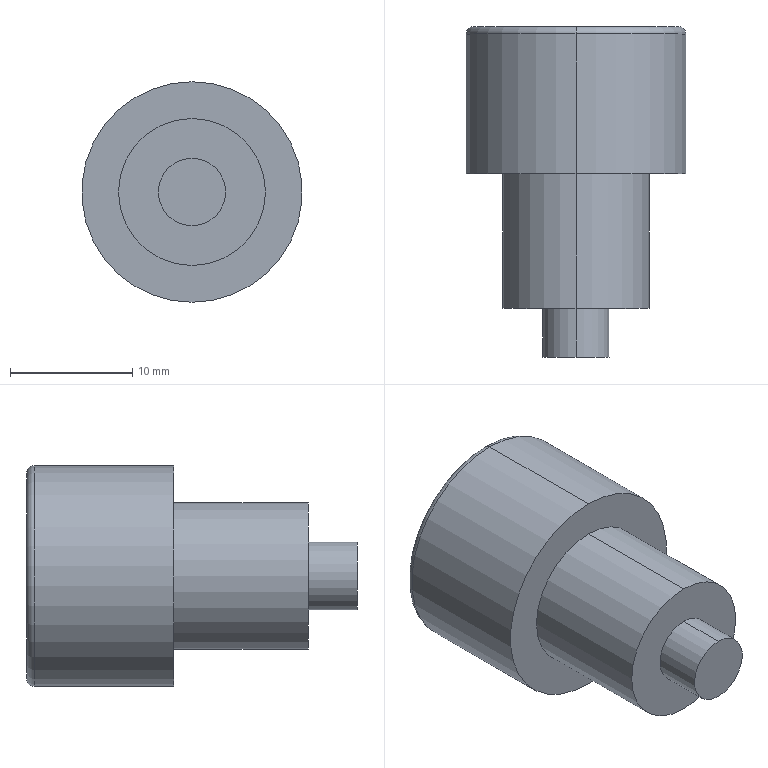Part | STEP file | Hex socket bolt M12x10 | 1 solid | 19 faces | box 18 x 27 x 18 mm | volume 3856 mm3 | plane 11 | cylinder 6 | torus 2 | commonest cylinder face diameters 5.5 x2 12 x2 18 x2
STEP:
#1=CARTESIAN_POINT('',(0.,-11.,-2.75));
#2=VERTEX_POINT('',#1);
#3=CARTESIAN_POINT('',(0.,-11.,2.75));
#4=VERTEX_POINT('',#3);
#5=CARTESIAN_POINT('',(0.,-11.,0.));
#6=DIRECTION('',(0.,-1.,0.));
#7=DIRECTION('',(0.,0.,-1.));
#8=AXIS2_PLACEMENT_3D('',#5,#6,#7);
#9=CIRCLE('',#8,2.75);
#10=EDGE_CURVE('',#2,#4,#9,.T.);
#11=ORIENTED_EDGE('',*,*,#10,.T.);
#12=CARTESIAN_POINT('',(0.,-15.,2.75));
#13=VERTEX_POINT('',#12);
#14=CARTESIAN_POINT('',(0.,-11.,2.75));
#15=DIRECTION('',(0.,-1.,0.));
#16=VECTOR('',#15,1000.);
#17=LINE('',#14,#16);
#18=EDGE_CURVE('',#4,#13,#17,.T.);
#19=ORIENTED_EDGE('',*,*,#18,.T.);
#20=CARTESIAN_POINT('',(0.,-15.,-2.75));
#21=VERTEX_POINT('',#20);
#22=CARTESIAN_POINT('',(0.,-15.,0.));
#23=DIRECTION('',(0.,-1.,0.));
#24=DIRECTION('',(0.,0.,-1.));
#25=AXIS2_PLACEMENT_3D('',#22,#23,#24);
#26=CIRCLE('',#25,2.75);
#27=EDGE_CURVE('',#21,#13,#26,.T.);
#28=ORIENTED_EDGE('',*,*,#27,.F.);
#29=CARTESIAN_POINT('',(0.,-11.,-2.75));
#30=DIRECTION('',(0.,-1.,0.));
#31=VECTOR('',#30,1000.);
#32=LINE('',#29,#31);
#33=EDGE_CURVE('',#2,#21,#32,.T.);
#34=ORIENTED_EDGE('',*,*,#33,.F.);
#35=EDGE_LOOP('',(#11,#19,#28,#34));
#36=FACE_OUTER_BOUND('',#35,.T.);
#37=CARTESIAN_POINT('',(0.,-11.,0.));
#38=DIRECTION('',(0.,-1.,0.));
#39=DIRECTION('',(0.,0.,-1.));
#40=AXIS2_PLACEMENT_3D('',#37,#38,#39);
#41=CYLINDRICAL_SURFACE('',#40,2.75);
#42=ADVANCED_FACE('',(#36),#41,.T.);
#43=CARTESIAN_POINT('',(0.,11.4,-9.));
#44=VERTEX_POINT('',#43);
#45=CARTESIAN_POINT('',(0.,11.4,9.));
#46=VERTEX_POINT('',#45);
#47=CARTESIAN_POINT('',(0.,11.4,0.));
#48=DIRECTION('',(0.,-1.,0.));
#49=DIRECTION('',(0.,0.,1.));
#50=AXIS2_PLACEMENT_3D('',#47,#48,#49);
#51=CIRCLE('',#50,9.);
#52=EDGE_CURVE('',#44,#46,#51,.T.);
#53=ORIENTED_EDGE('',*,*,#52,.F.);
#54=CARTESIAN_POINT('',(0.,12.,-8.4));
#55=VERTEX_POINT('',#54);
#56=CARTESIAN_POINT('',(0.,11.4,-8.4));
#57=DIRECTION('',(1.,0.,0.));
#58=DIRECTION('',(0.,0.,-1.));
#59=AXIS2_PLACEMENT_3D('',#56,#57,#58);
#60=CIRCLE('',#59,0.6);
#61=EDGE_CURVE('',#44,#55,#60,.T.);
#62=ORIENTED_EDGE('',*,*,#61,.T.);
#63=CARTESIAN_POINT('',(0.,12.,8.4));
#64=VERTEX_POINT('',#63);
#65=CARTESIAN_POINT('',(0.,12.,0.));
#66=DIRECTION('',(0.,1.,0.));
#67=DIRECTION('',(0.,0.,1.));
#68=AXIS2_PLACEMENT_3D('',#65,#66,#67);
#69=CIRCLE('',#68,8.4);
#70=EDGE_CURVE('',#64,#55,#69,.T.);
#71=ORIENTED_EDGE('',*,*,#70,.F.);
#72=CARTESIAN_POINT('',(0.,11.4,8.4));
#73=DIRECTION('',(-1.,0.,0.));
#74=DIRECTION('',(0.,0.,1.));
#75=AXIS2_PLACEMENT_3D('',#72,#73,#74);
#76=CIRCLE('',#75,0.6);
#77=EDGE_CURVE('',#46,#64,#76,.T.);
#78=ORIENTED_EDGE('',*,*,#77,.F.);
#79=EDGE_LOOP('',(#53,#62,#71,#78));
#80=FACE_OUTER_BOUND('',#79,.T.);
#81=CARTESIAN_POINT('',(0.,11.4,0.));
#82=DIRECTION('',(0.,1.,0.));
#83=DIRECTION('',(0.,0.,1.));
#84=AXIS2_PLACEMENT_3D('',#81,#82,#83);
#85=TOROIDAL_SURFACE('',#84,8.4,0.6);
#86=ADVANCED_FACE('',(#80),#85,.T.);
#87=ORIENTED_EDGE('',*,*,#52,.T.);
#88=CARTESIAN_POINT('',(0.,0.,9.));
#89=VERTEX_POINT('',#88);
#90=CARTESIAN_POINT('',(0.,12.,9.));
#91=DIRECTION('',(0.,-1.,0.));
#92=VECTOR('',#91,1000.);
#93=LINE('',#90,#92);
#94=EDGE_CURVE('',#46,#89,#93,.T.);
#95=ORIENTED_EDGE('',*,*,#94,.T.);
#96=CARTESIAN_POINT('',(0.,0.,-9.));
#97=VERTEX_POINT('',#96);
#98=CARTESIAN_POINT('',(0.,0.,0.));
#99=DIRECTION('',(0.,1.,0.));
#100=DIRECTION('',(0.,0.,1.));
#101=AXIS2_PLACEMENT_3D('',#98,#99,#100);
#102=CIRCLE('',#101,9.);
#103=EDGE_CURVE('',#89,#97,#102,.T.);
#104=ORIENTED_EDGE('',*,*,#103,.T.);
#105=CARTESIAN_POINT('',(0.,12.,-9.));
#106=DIRECTION('',(0.,-1.,0.));
#107=VECTOR('',#106,1000.);
#108=LINE('',#105,#107);
#109=EDGE_CURVE('',#44,#97,#108,.T.);
#110=ORIENTED_EDGE('',*,*,#109,.F.);
#111=EDGE_LOOP('',(#87,#95,#104,#110));
#112=FACE_OUTER_BOUND('',#111,.T.);
#113=CARTESIAN_POINT('',(0.,12.,0.));
#114=DIRECTION('',(0.,-1.,0.));
#115=DIRECTION('',(0.,0.,-1.));
#116=AXIS2_PLACEMENT_3D('',#113,#114,#115);
#117=CYLINDRICAL_SURFACE('',#116,9.);
#118=ADVANCED_FACE('',(#112),#117,.T.);
#119=CARTESIAN_POINT('',(0.,-11.,-6.));
#120=VERTEX_POINT('',#119);
#121=CARTESIAN_POINT('',(0.,-11.,6.));
#122=VERTEX_POINT('',#121);
#123=CARTESIAN_POINT('',(0.,-11.,0.));
#124=DIRECTION('',(0.,-1.,0.));
#125=DIRECTION('',(0.,0.,-1.));
#126=AXIS2_PLACEMENT_3D('',#123,#124,#125);
#127=CIRCLE('',#126,6.);
#128=EDGE_CURVE('',#120,#122,#127,.T.);
#129=ORIENTED_EDGE('',*,*,#128,.F.);
#130=CARTESIAN_POINT('',(0.,0.,-6.));
#131=VERTEX_POINT('',#130);
#132=CARTESIAN_POINT('',(0.,-15.,-6.));
#133=DIRECTION('',(0.,1.,0.));
#134=VECTOR('',#133,1000.);
#135=LINE('',#132,#134);
#136=EDGE_CURVE('',#120,#131,#135,.T.);
#137=ORIENTED_EDGE('',*,*,#136,.T.);
#138=CARTESIAN_POINT('',(0.,0.,6.));
#139=VERTEX_POINT('',#138);
#140=CARTESIAN_POINT('',(0.,0.,0.));
#141=DIRECTION('',(0.,-1.,0.));
#142=DIRECTION('',(0.,0.,1.));
#143=AXIS2_PLACEMENT_3D('',#140,#141,#142);
#144=CIRCLE('',#143,6.);
#145=EDGE_CURVE('',#131,#139,#144,.T.);
#146=ORIENTED_EDGE('',*,*,#145,.T.);
#147=CARTESIAN_POINT('',(0.,-15.,6.));
#148=DIRECTION('',(0.,1.,0.));
#149=VECTOR('',#148,1000.);
#150=LINE('',#147,#149);
#151=EDGE_CURVE('',#122,#139,#150,.T.);
#152=ORIENTED_EDGE('',*,*,#151,.F.);
#153=EDGE_LOOP('',(#129,#137,#146,#152));
#154=FACE_OUTER_BOUND('',#153,.T.);
#155=CARTESIAN_POINT('',(0.,-15.,0.));
#156=DIRECTION('',(0.,1.,0.));
#157=DIRECTION('',(0.,0.,1.));
#158=AXIS2_PLACEMENT_3D('',#155,#156,#157);
#159=CYLINDRICAL_SURFACE('',#158,6.);
#160=ADVANCED_FACE('',(#154),#159,.T.);
#161=ORIENTED_EDGE('',*,*,#136,.F.);
#162=CARTESIAN_POINT('',(0.,-11.,0.));
#163=DIRECTION('',(0.,-1.,0.));
#164=DIRECTION('',(0.,0.,-1.));
#165=AXIS2_PLACEMENT_3D('',#162,#163,#164);
#166=CIRCLE('',#165,6.);
#167=EDGE_CURVE('',#122,#120,#166,.T.);
#168=ORIENTED_EDGE('',*,*,#167,.F.);
#169=ORIENTED_EDGE('',*,*,#151,.T.);
#170=CARTESIAN_POINT('',(0.,0.,0.));
#171=DIRECTION('',(0.,-1.,0.));
#172=DIRECTION('',(0.,0.,1.));
#173=AXIS2_PLACEMENT_3D('',#170,#171,#172);
#174=CIRCLE('',#173,6.);
#175=EDGE_CURVE('',#139,#131,#174,.T.);
#176=ORIENTED_EDGE('',*,*,#175,.T.);
#177=EDGE_LOOP('',(#161,#168,#169,#176));
#178=FACE_OUTER_BOUND('',#177,.T.);
#179=CARTESIAN_POINT('',(0.,-15.,0.));
#180=DIRECTION('',(0.,1.,0.));
#181=DIRECTION('',(0.,0.,1.));
#182=AXIS2_PLACEMENT_3D('',#179,#180,#181);
#183=CYLINDRICAL_SURFACE('',#182,6.);
#184=ADVANCED_FACE('',(#178),#183,.T.);
#185=CARTESIAN_POINT('',(0.,0.,0.));
#186=DIRECTION('',(0.,1.,0.));
#187=DIRECTION('',(0.,0.,1.));
#188=AXIS2_PLACEMENT_3D('',#185,#186,#187);
#189=CIRCLE('',#188,9.);
#190=EDGE_CURVE('',#97,#89,#189,.T.);
#191=ORIENTED_EDGE('',*,*,#190,.F.);
#192=ORIENTED_EDGE('',*,*,#103,.F.);
#193=EDGE_LOOP('',(#191,#192));
#194=FACE_OUTER_BOUND('',#193,.T.);
#195=ORIENTED_EDGE('',*,*,#175,.F.);
#196=ORIENTED_EDGE('',*,*,#145,.F.);
#197=EDGE_LOOP('',(#195,#196));
#198=FACE_BOUND('',#197,.T.);
#199=CARTESIAN_POINT('',(0.,0.,0.));
#200=DIRECTION('',(0.,1.,0.));
#201=DIRECTION('',(0.,0.,1.));
#202=AXIS2_PLACEMENT_3D('',#199,#200,#201);
#203=PLANE('',#202);
#204=ADVANCED_FACE('',(#194,#198),#203,.F.);
#205=ORIENTED_EDGE('',*,*,#94,.F.);
#206=CARTESIAN_POINT('',(0.,11.4,0.));
#207=DIRECTION('',(0.,-1.,0.));
#208=DIRECTION('',(0.,0.,1.));
#209=AXIS2_PLACEMENT_3D('',#206,#207,#208);
#210=CIRCLE('',#209,9.);
#211=EDGE_CURVE('',#46,#44,#210,.T.);
#212=ORIENTED_EDGE('',*,*,#211,.T.);
#213=ORIENTED_EDGE('',*,*,#109,.T.);
#214=ORIENTED_EDGE('',*,*,#190,.T.);
#215=EDGE_LOOP('',(#205,#212,#213,#214));
#216=FACE_OUTER_BOUND('',#215,.T.);
#217=CARTESIAN_POINT('',(0.,12.,0.));
#218=DIRECTION('',(0.,-1.,0.));
#219=DIRECTION('',(0.,0.,-1.));
#220=AXIS2_PLACEMENT_3D('',#217,#218,#219);
#221=CYLINDRICAL_SURFACE('',#220,9.);
#222=ADVANCED_FACE('',(#216),#221,.T.);
#223=ORIENTED_EDGE('',*,*,#70,.T.);
#224=CARTESIAN_POINT('',(0.,12.,0.));
#225=DIRECTION('',(0.,1.,0.));
#226=DIRECTION('',(0.,0.,1.));
#227=AXIS2_PLACEMENT_3D('',#224,#225,#226);
#228=CIRCLE('',#227,8.4);
#229=EDGE_CURVE('',#55,#64,#228,.T.);
#230=ORIENTED_EDGE('',*,*,#229,.T.);
#231=EDGE_LOOP('',(#223,#230));
#232=FACE_OUTER_BOUND('',#231,.T.);
#233=CARTESIAN_POINT('',(2.921,12.,5.06));
#234=VERTEX_POINT('',#233);
#235=CARTESIAN_POINT('',(5.843,12.,0.));
#236=VERTEX_POINT('',#235);
#237=CARTESIAN_POINT('',(2.921,12.,5.06));
#238=DIRECTION('',(0.5,0.,-0.866));
#239=VECTOR('',#238,1000.);
#240=LINE('',#237,#239);
#241=EDGE_CURVE('',#234,#236,#240,.T.);
#242=ORIENTED_EDGE('',*,*,#241,.F.);
#243=CARTESIAN_POINT('',(-2.921,12.,5.06));
#244=VERTEX_POINT('',#243);
#245=CARTESIAN_POINT('',(-2.921,12.,5.06));
#246=DIRECTION('',(1.,0.,0.));
#247=VECTOR('',#246,1000.);
#248=LINE('',#245,#247);
#249=EDGE_CURVE('',#244,#234,#248,.T.);
#250=ORIENTED_EDGE('',*,*,#249,.F.);
#251=CARTESIAN_POINT('',(-5.843,12.,0.));
#252=VERTEX_POINT('',#251);
#253=CARTESIAN_POINT('',(-5.843,12.,0.));
#254=DIRECTION('',(0.5,0.,0.866));
#255=VECTOR('',#254,1000.);
#256=LINE('',#253,#255);
#257=EDGE_CURVE('',#252,#244,#256,.T.);
#258=ORIENTED_EDGE('',*,*,#257,.F.);
#259=CARTESIAN_POINT('',(-2.921,12.,-5.06));
#260=VERTEX_POINT('',#259);
#261=CARTESIAN_POINT('',(-2.921,12.,-5.06));
#262=DIRECTION('',(-0.5,0.,0.866));
#263=VECTOR('',#262,1000.);
#264=LINE('',#261,#263);
#265=EDGE_CURVE('',#260,#252,#264,.T.);
#266=ORIENTED_EDGE('',*,*,#265,.F.);
#267=CARTESIAN_POINT('',(2.921,12.,-5.06));
#268=VERTEX_POINT('',#267);
#269=CARTESIAN_POINT('',(2.921,12.,-5.06));
#270=DIRECTION('',(-1.,0.,0.));
#271=VECTOR('',#270,1000.);
#272=LINE('',#269,#271);
#273=EDGE_CURVE('',#268,#260,#272,.T.);
#274=ORIENTED_EDGE('',*,*,#273,.F.);
#275=CARTESIAN_POINT('',(5.843,12.,0.));
#276=DIRECTION('',(-0.5,0.,-0.866));
#277=VECTOR('',#276,1000.);
#278=LINE('',#275,#277);
#279=EDGE_CURVE('',#236,#268,#278,.T.);
#280=ORIENTED_EDGE('',*,*,#279,.F.);
#281=EDGE_LOOP('',(#242,#250,#258,#266,#274,#280));
#282=FACE_BOUND('',#281,.T.);
#283=CARTESIAN_POINT('',(0.,12.,0.));
#284=DIRECTION('',(0.,1.,0.));
#285=DIRECTION('',(0.,0.,1.));
#286=AXIS2_PLACEMENT_3D('',#283,#284,#285);
#287=PLANE('',#286);
#288=ADVANCED_FACE('',(#232,#282),#287,.T.);
#289=ORIENTED_EDGE('',*,*,#241,.T.);
#290=CARTESIAN_POINT('',(5.843,6.,0.));
#291=VERTEX_POINT('',#290);
#292=CARTESIAN_POINT('',(5.843,6.,0.));
#293=DIRECTION('',(0.,1.,0.));
#294=VECTOR('',#293,1000.);
#295=LINE('',#292,#294);
#296=EDGE_CURVE('',#291,#236,#295,.T.);
#297=ORIENTED_EDGE('',*,*,#296,.F.);
#298=CARTESIAN_POINT('',(2.921,6.,5.06));
#299=VERTEX_POINT('',#298);
#300=CARTESIAN_POINT('',(2.921,6.,5.06));
#301=DIRECTION('',(0.5,0.,-0.866));
#302=VECTOR('',#301,1000.);
#303=LINE('',#300,#302);
#304=EDGE_CURVE('',#299,#291,#303,.T.);
#305=ORIENTED_EDGE('',*,*,#304,.F.);
#306=CARTESIAN_POINT('',(2.921,6.,5.06));
#307=DIRECTION('',(0.,1.,0.));
#308=VECTOR('',#307,1000.);
#309=LINE('',#306,#308);
#310=EDGE_CURVE('',#299,#234,#309,.T.);
#311=ORIENTED_EDGE('',*,*,#310,.T.);
#312=EDGE_LOOP('',(#289,#297,#305,#311));
#313=FACE_OUTER_BOUND('',#312,.T.);
#314=CARTESIAN_POINT('',(2.921,6.,5.06));
#315=DIRECTION('',(0.866,0.,0.5));
#316=DIRECTION('',(0.5,0.,-0.866));
#317=AXIS2_PLACEMENT_3D('',#314,#315,#316);
#318=PLANE('',#317);
#319=ADVANCED_FACE('',(#313),#318,.F.);
#320=ORIENTED_EDGE('',*,*,#249,.T.);
#321=ORIENTED_EDGE('',*,*,#310,.F.);
#322=CARTESIAN_POINT('',(-2.921,6.,5.06));
#323=VERTEX_POINT('',#322);
#324=CARTESIAN_POINT('',(-2.921,6.,5.06));
#325=DIRECTION('',(1.,0.,0.));
#326=VECTOR('',#325,1000.);
#327=LINE('',#324,#326);
#328=EDGE_CURVE('',#323,#299,#327,.T.);
#329=ORIENTED_EDGE('',*,*,#328,.F.);
#330=CARTESIAN_POINT('',(-2.921,6.,5.06));
#331=DIRECTION('',(0.,1.,0.));
#332=VECTOR('',#331,1000.);
#333=LINE('',#330,#332);
#334=EDGE_CURVE('',#323,#244,#333,.T.);
#335=ORIENTED_EDGE('',*,*,#334,.T.);
#336=EDGE_LOOP('',(#320,#321,#329,#335));
#337=FACE_OUTER_BOUND('',#336,.T.);
#338=CARTESIAN_POINT('',(-2.921,6.,5.06));
#339=DIRECTION('',(0.,0.,1.));
#340=DIRECTION('',(1.,0.,0.));
#341=AXIS2_PLACEMENT_3D('',#338,#339,#340);
#342=PLANE('',#341);
#343=ADVANCED_FACE('',(#337),#342,.F.);
#344=ORIENTED_EDGE('',*,*,#257,.T.);
#345=ORIENTED_EDGE('',*,*,#334,.F.);
#346=CARTESIAN_POINT('',(-5.843,6.,0.));
#347=VERTEX_POINT('',#346);
#348=CARTESIAN_POINT('',(-5.843,6.,0.));
#349=DIRECTION('',(0.5,0.,0.866));
#350=VECTOR('',#349,1000.);
#351=LINE('',#348,#350);
#352=EDGE_CURVE('',#347,#323,#351,.T.);
#353=ORIENTED_EDGE('',*,*,#352,.F.);
#354=CARTESIAN_POINT('',(-5.843,6.,0.));
#355=DIRECTION('',(0.,1.,0.));
#356=VECTOR('',#355,1000.);
#357=LINE('',#354,#356);
#358=EDGE_CURVE('',#347,#252,#357,.T.);
#359=ORIENTED_EDGE('',*,*,#358,.T.);
#360=EDGE_LOOP('',(#344,#345,#353,#359));
#361=FACE_OUTER_BOUND('',#360,.T.);
#362=CARTESIAN_POINT('',(-5.843,6.,0.));
#363=DIRECTION('',(-0.866,0.,0.5));
#364=DIRECTION('',(0.5,0.,0.866));
#365=AXIS2_PLACEMENT_3D('',#362,#363,#364);
#366=PLANE('',#365);
#367=ADVANCED_FACE('',(#361),#366,.F.);
#368=ORIENTED_EDGE('',*,*,#265,.T.);
#369=ORIENTED_EDGE('',*,*,#358,.F.);
#370=CARTESIAN_POINT('',(-2.921,6.,-5.06));
#371=VERTEX_POINT('',#370);
#372=CARTESIAN_POINT('',(-2.921,6.,-5.06));
#373=DIRECTION('',(-0.5,0.,0.866));
#374=VECTOR('',#373,1000.);
#375=LINE('',#372,#374);
#376=EDGE_CURVE('',#371,#347,#375,.T.);
#377=ORIENTED_EDGE('',*,*,#376,.F.);
#378=CARTESIAN_POINT('',(-2.921,6.,-5.06));
#379=DIRECTION('',(0.,1.,0.));
#380=VECTOR('',#379,1000.);
#381=LINE('',#378,#380);
#382=EDGE_CURVE('',#371,#260,#381,.T.);
#383=ORIENTED_EDGE('',*,*,#382,.T.);
#384=EDGE_LOOP('',(#368,#369,#377,#383));
#385=FACE_OUTER_BOUND('',#384,.T.);
#386=CARTESIAN_POINT('',(-2.921,6.,-5.06));
#387=DIRECTION('',(-0.866,0.,-0.5));
#388=DIRECTION('',(-0.5,0.,0.866));
#389=AXIS2_PLACEMENT_3D('',#386,#387,#388);
#390=PLANE('',#389);
#391=ADVANCED_FACE('',(#385),#390,.F.);
#392=ORIENTED_EDGE('',*,*,#273,.T.);
#393=ORIENTED_EDGE('',*,*,#382,.F.);
#394=CARTESIAN_POINT('',(2.921,6.,-5.06));
#395=VERTEX_POINT('',#394);
#396=CARTESIAN_POINT('',(2.921,6.,-5.06));
#397=DIRECTION('',(-1.,0.,0.));
#398=VECTOR('',#397,1000.);
#399=LINE('',#396,#398);
#400=EDGE_CURVE('',#395,#371,#399,.T.);
#401=ORIENTED_EDGE('',*,*,#400,.F.);
#402=CARTESIAN_POINT('',(2.921,6.,-5.06));
#403=DIRECTION('',(0.,1.,0.));
#404=VECTOR('',#403,1000.);
#405=LINE('',#402,#404);
#406=EDGE_CURVE('',#395,#268,#405,.T.);
#407=ORIENTED_EDGE('',*,*,#406,.T.);
#408=EDGE_LOOP('',(#392,#393,#401,#407));
#409=FACE_OUTER_BOUND('',#408,.T.);
#410=CARTESIAN_POINT('',(2.921,6.,-5.06));
#411=DIRECTION('',(0.,0.,-1.));
#412=DIRECTION('',(-1.,0.,0.));
#413=AXIS2_PLACEMENT_3D('',#410,#411,#412);
#414=PLANE('',#413);
#415=ADVANCED_FACE('',(#409),#414,.F.);
#416=ORIENTED_EDGE('',*,*,#279,.T.);
#417=ORIENTED_EDGE('',*,*,#406,.F.);
#418=CARTESIAN_POINT('',(5.843,6.,0.));
#419=DIRECTION('',(-0.5,0.,-0.866));
#420=VECTOR('',#419,1000.);
#421=LINE('',#418,#420);
#422=EDGE_CURVE('',#291,#395,#421,.T.);
#423=ORIENTED_EDGE('',*,*,#422,.F.);
#424=ORIENTED_EDGE('',*,*,#296,.T.);
#425=EDGE_LOOP('',(#416,#417,#423,#424));
#426=FACE_OUTER_BOUND('',#425,.T.);
#427=CARTESIAN_POINT('',(5.843,6.,0.));
#428=DIRECTION('',(0.866,0.,-0.5));
#429=DIRECTION('',(-0.5,0.,-0.866));
#430=AXIS2_PLACEMENT_3D('',#427,#428,#429);
#431=PLANE('',#430);
#432=ADVANCED_FACE('',(#426),#431,.F.);
#433=ORIENTED_EDGE('',*,*,#304,.T.);
#434=ORIENTED_EDGE('',*,*,#422,.T.);
#435=ORIENTED_EDGE('',*,*,#400,.T.);
#436=ORIENTED_EDGE('',*,*,#376,.T.);
#437=ORIENTED_EDGE('',*,*,#352,.T.);
#438=ORIENTED_EDGE('',*,*,#328,.T.);
#439=EDGE_LOOP('',(#433,#434,#435,#436,#437,#438));
#440=FACE_OUTER_BOUND('',#439,.T.);
#441=CARTESIAN_POINT('',(0.,6.,0.));
#442=DIRECTION('',(0.,1.,0.));
#443=DIRECTION('',(0.,0.,1.));
#444=AXIS2_PLACEMENT_3D('',#441,#442,#443);
#445=PLANE('',#444);
#446=ADVANCED_FACE('',(#440),#445,.T.);
#447=ORIENTED_EDGE('',*,*,#61,.F.);
#448=ORIENTED_EDGE('',*,*,#211,.F.);
#449=ORIENTED_EDGE('',*,*,#77,.T.);
#450=ORIENTED_EDGE('',*,*,#229,.F.);
#451=EDGE_LOOP('',(#447,#448,#449,#450));
#452=FACE_OUTER_BOUND('',#451,.T.);
#453=CARTESIAN_POINT('',(0.,11.4,0.));
#454=DIRECTION('',(0.,1.,0.));
#455=DIRECTION('',(0.,0.,1.));
#456=AXIS2_PLACEMENT_3D('',#453,#454,#455);
#457=TOROIDAL_SURFACE('',#456,8.4,0.6);
#458=ADVANCED_FACE('',(#452),#457,.T.);
#459=ORIENTED_EDGE('',*,*,#10,.F.);
#460=CARTESIAN_POINT('',(0.,-11.,0.));
#461=DIRECTION('',(0.,-1.,0.));
#462=DIRECTION('',(0.,0.,-1.));
#463=AXIS2_PLACEMENT_3D('',#460,#461,#462);
#464=CIRCLE('',#463,2.75);
#465=EDGE_CURVE('',#4,#2,#464,.T.);
#466=ORIENTED_EDGE('',*,*,#465,.F.);
#467=EDGE_LOOP('',(#459,#466));
#468=FACE_BOUND('',#467,.T.);
#469=ORIENTED_EDGE('',*,*,#167,.T.);
#470=ORIENTED_EDGE('',*,*,#128,.T.);
#471=EDGE_LOOP('',(#469,#470));
#472=FACE_OUTER_BOUND('',#471,.T.);
#473=CARTESIAN_POINT('',(0.,-11.,0.));
#474=DIRECTION('',(0.,-1.,0.));
#475=DIRECTION('',(0.,0.,-1.));
#476=AXIS2_PLACEMENT_3D('',#473,#474,#475);
#477=PLANE('',#476);
#478=ADVANCED_FACE('',(#468,#472),#477,.T.);
#479=ORIENTED_EDGE('',*,*,#18,.F.);
#480=ORIENTED_EDGE('',*,*,#465,.T.);
#481=ORIENTED_EDGE('',*,*,#33,.T.);
#482=CARTESIAN_POINT('',(0.,-15.,0.));
#483=DIRECTION('',(0.,-1.,0.));
#484=DIRECTION('',(0.,0.,-1.));
#485=AXIS2_PLACEMENT_3D('',#482,#483,#484);
#486=CIRCLE('',#485,2.75);
#487=EDGE_CURVE('',#13,#21,#486,.T.);
#488=ORIENTED_EDGE('',*,*,#487,.F.);
#489=EDGE_LOOP('',(#479,#480,#481,#488));
#490=FACE_OUTER_BOUND('',#489,.T.);
#491=CARTESIAN_POINT('',(0.,-11.,0.));
#492=DIRECTION('',(0.,-1.,0.));
#493=DIRECTION('',(0.,0.,-1.));
#494=AXIS2_PLACEMENT_3D('',#491,#492,#493);
#495=CYLINDRICAL_SURFACE('',#494,2.75);
#496=ADVANCED_FACE('',(#490),#495,.T.);
#497=ORIENTED_EDGE('',*,*,#27,.T.);
#498=ORIENTED_EDGE('',*,*,#487,.T.);
#499=EDGE_LOOP('',(#497,#498));
#500=FACE_OUTER_BOUND('',#499,.T.);
#501=CARTESIAN_POINT('',(0.,-15.,0.));
#502=DIRECTION('',(0.,-1.,0.));
#503=DIRECTION('',(0.,0.,-1.));
#504=AXIS2_PLACEMENT_3D('',#501,#502,#503);
#505=PLANE('',#504);
#506=ADVANCED_FACE('',(#500),#505,.T.);
#507=CLOSED_SHELL('',(#42,#86,#118,#160,#184,#204,#222,#288,#319,#343,#367,#391,#415,#432,#446,#458,#478,#496,#506));
#508=MANIFOLD_SOLID_BREP('',#507);
#509=CARTESIAN_POINT('',(0.,0.,0.));
#510=DIRECTION('',(0.,0.,1.));
#511=DIRECTION('',(1.,0.,0.));
#512=AXIS2_PLACEMENT_3D('',#509,#510,#511);
#513=(LENGTH_UNIT()NAMED_UNIT(*)SI_UNIT(.MILLI.,.METRE.));
#514=UNCERTAINTY_MEASURE_WITH_UNIT(LENGTH_MEASURE(0.00001),#513,'','');
#515=(NAMED_UNIT(*)PLANE_ANGLE_UNIT()SI_UNIT($,.RADIAN.));
#516=(NAMED_UNIT(*)SI_UNIT($,.STERADIAN.)SOLID_ANGLE_UNIT());
#517=(GEOMETRIC_REPRESENTATION_CONTEXT(3)GLOBAL_UNCERTAINTY_ASSIGNED_CONTEXT((#514))GLOBAL_UNIT_ASSIGNED_CONTEXT((#513,#515,#516))REPRESENTATION_CONTEXT('',''));
#518=ADVANCED_BREP_SHAPE_REPRESENTATION('',(#508,#512),#517);